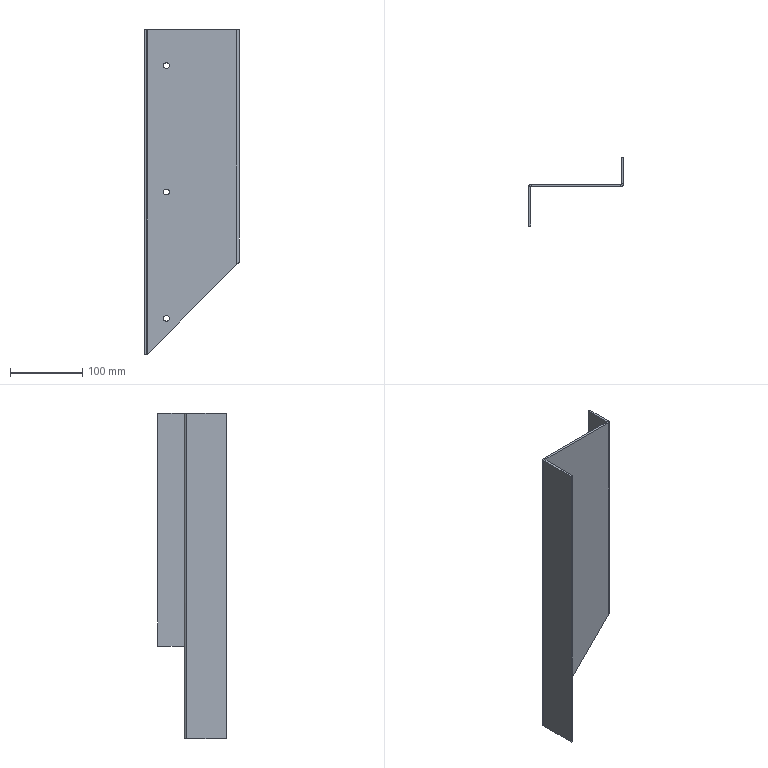Part | STEP file | TS-Z001-002 | 1 solid | 28 faces | box 131 x 95 x 450 mm | volume 260117 mm3 | plane 16 | cylinder 10 | spline 2 | commonest cylinder face diameters 8 x6 0.4 x2 6.4 x2